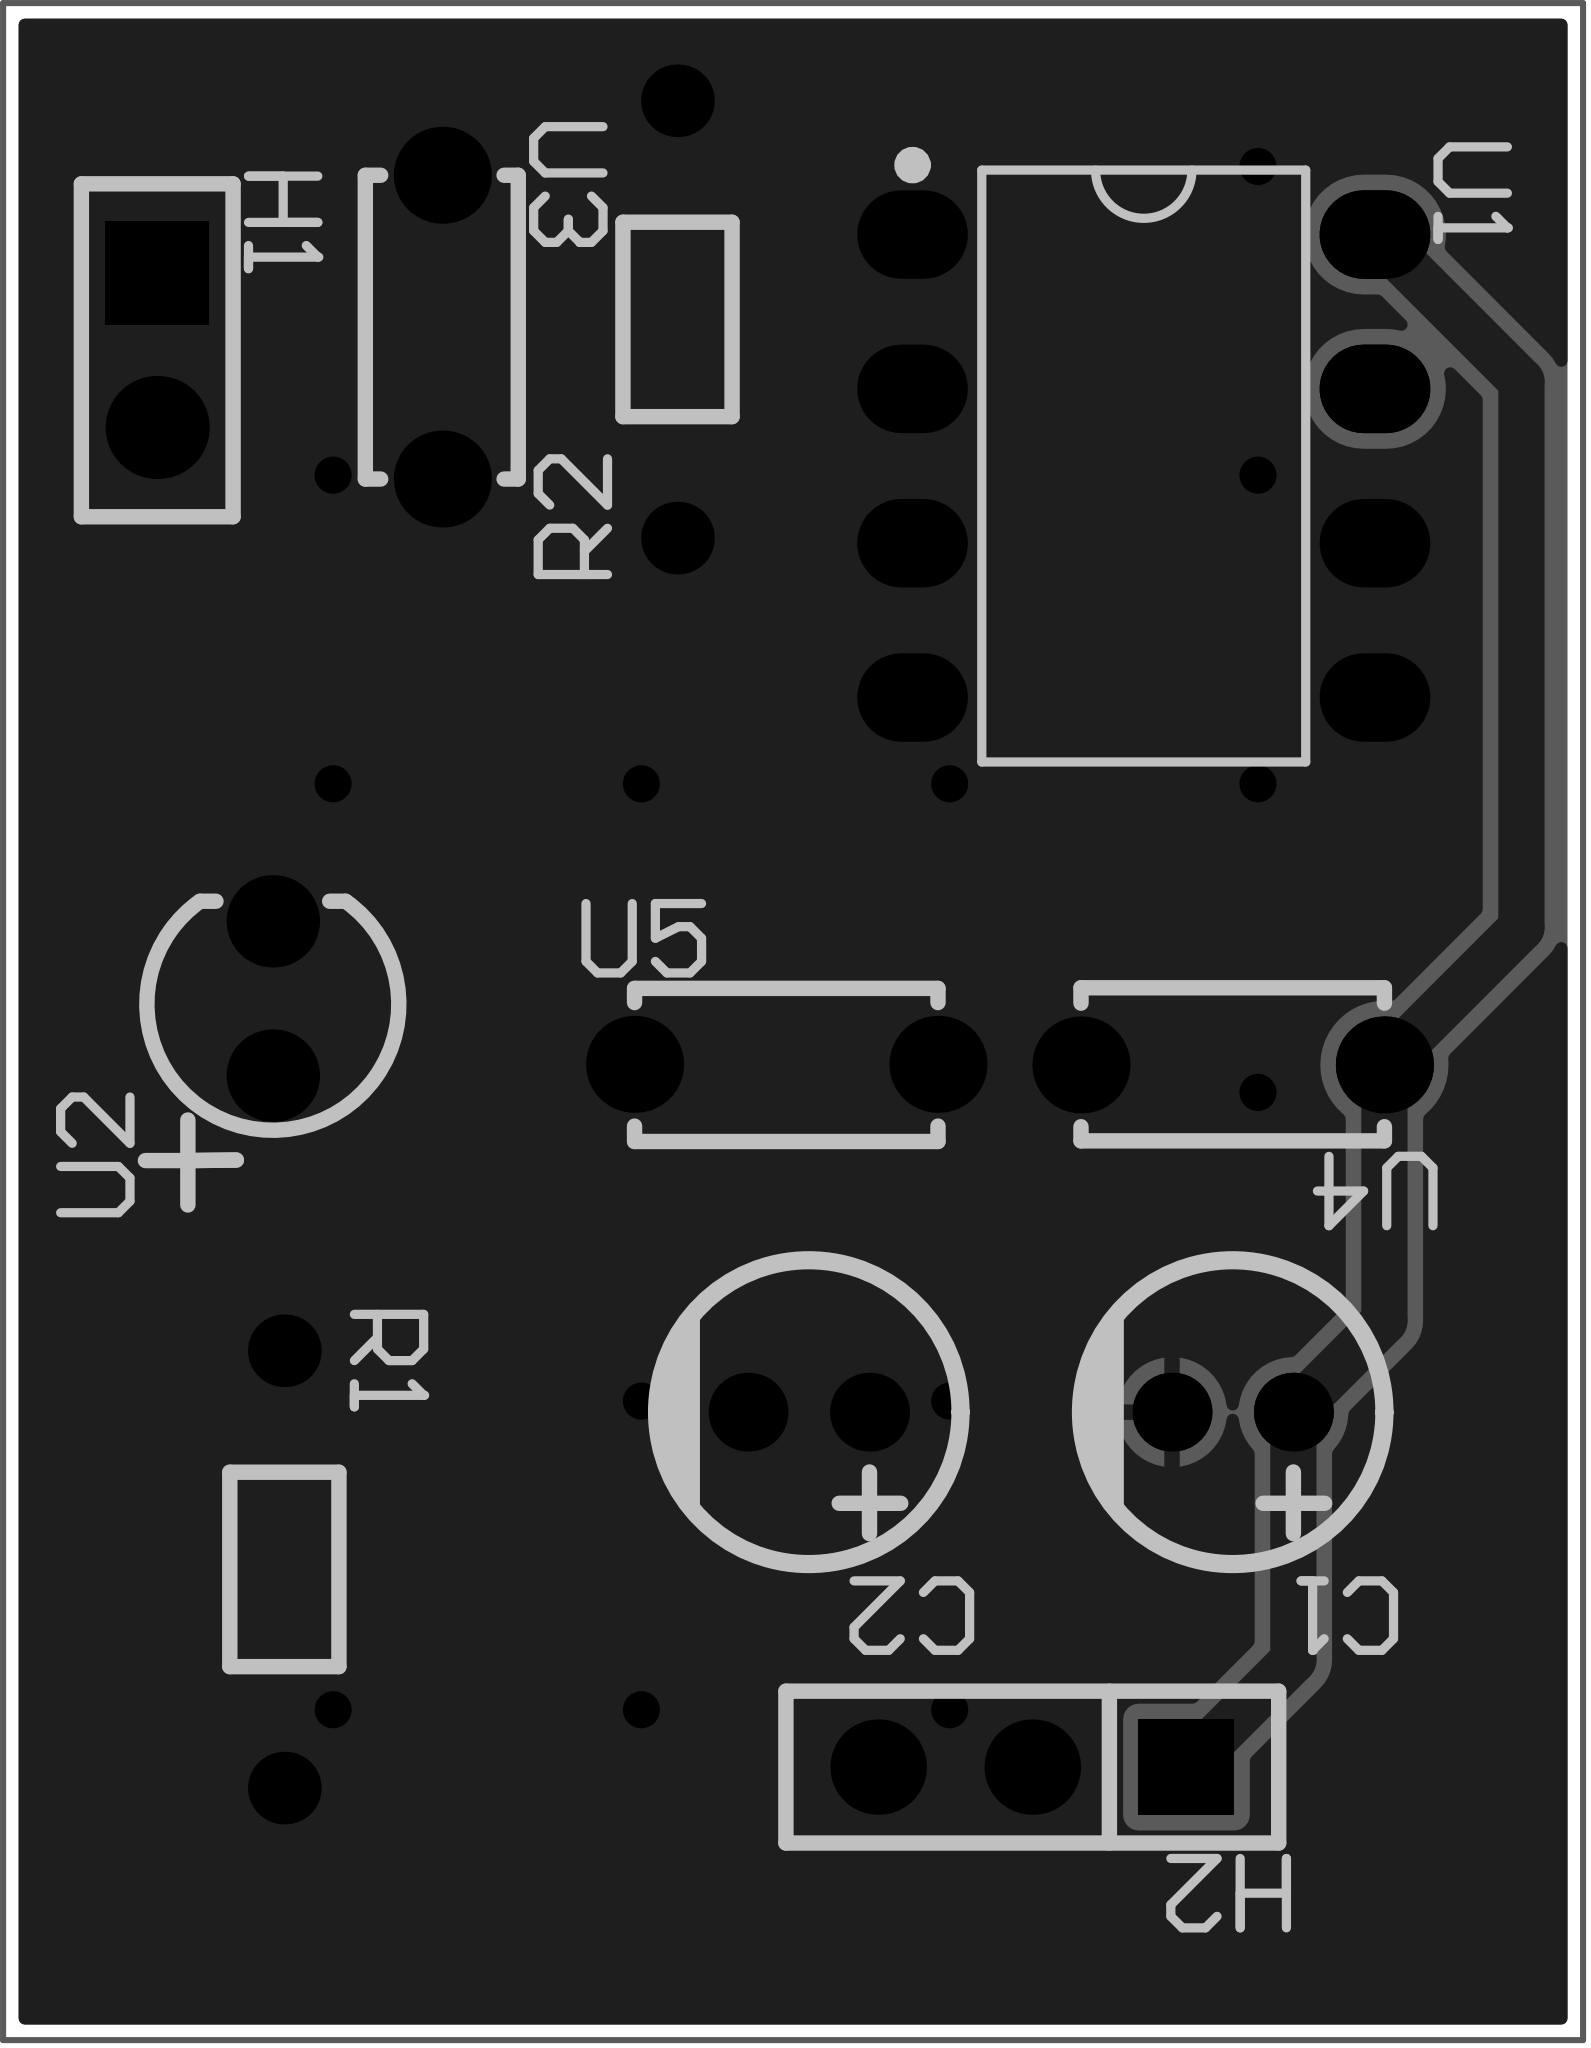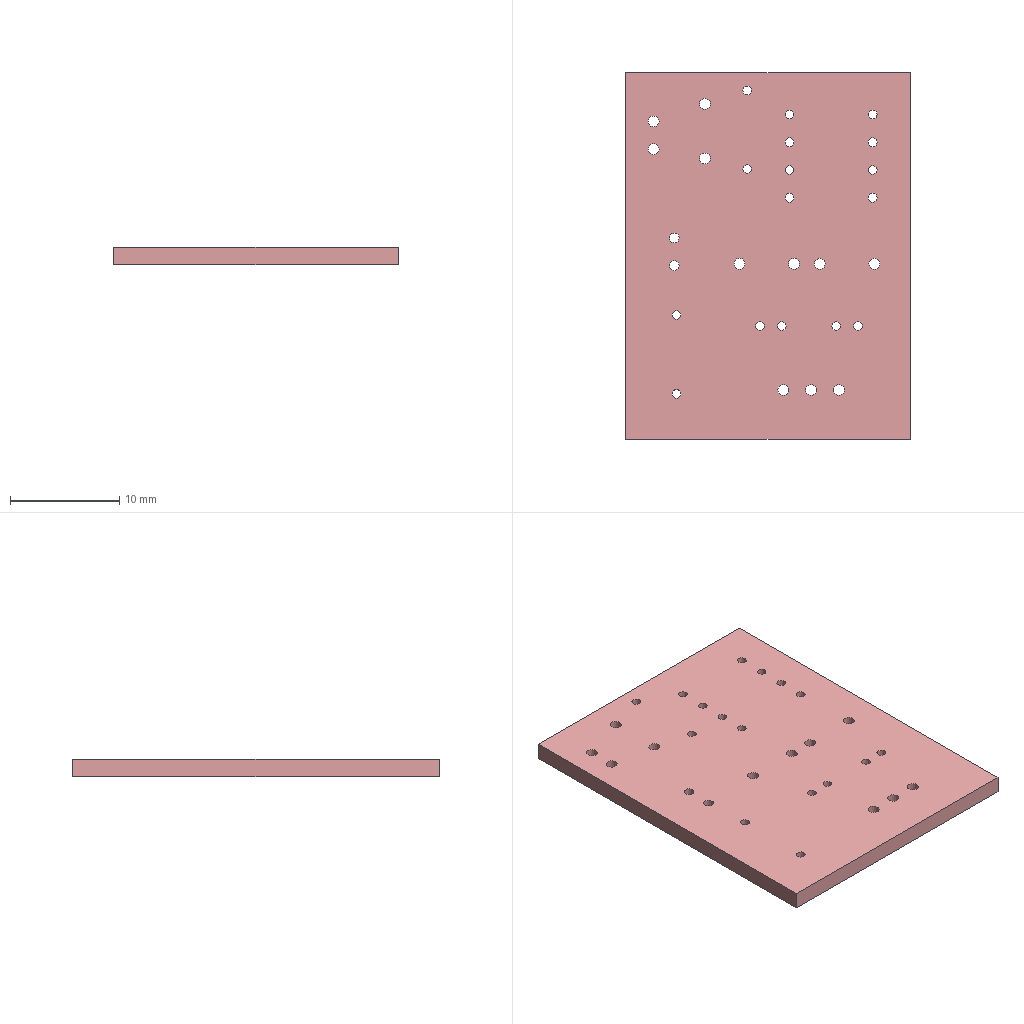Circuit board layout | Altium Designer | box 26 x 33.5 x 1.6 mm
Layer stack:
# Altium Designer layer stack of  (unit mm; dielectric type: 0 none, 1 core, 2 prepreg, 3 surface material)
index,name,kind,layer,copper_thickness_mm,dielectric_type,dielectric_thickness_mm,dielectric_material,dielectric_constant
0,Top Paste Mask Layer,other,,,,,,
1,Top Silkscreen Layer,other,,,,,,
2,Top Solder Mask Layer,dielectric,,,3,0.01,,3.3
3,Top Layer,copper,Top Layer,0.035,,,,
4,Dielectric1,dielectric,,,3,1.51,FR4,4.5
5,Bottom Layer,copper,Bottom Layer,0.035,,,,
6,Bottom Solder Mask Layer,dielectric,,,3,0.01,,3.3
7,Bottom Silkscreen Layer,other,,,,,,
8,Bottom Paste Mask Layer,other,,,,,,
# drill layer pairs: low layer,high layer
drill_pair,Top Layer,Bottom Layer
Part placement:
Designator,Comment,Layer,Footprint,Center-X(mm),Center-Y(mm),Rotation
C1,10uF,TopLayer,CAP-TH_BD5.0-P2.00-D0.8-FD-10UF50VC110GL,100.272,88.695,180
C2,10uF,TopLayer,CAP-TH_BD5.0-P2.00-D0.8-FD-10UF50VC110GL,93.287,88.695,180
H1,,TopLayer,HDR-TH_2P-P2.54-V-F,82.55,106.172,270
H2,,TopLayer,HDR-TH_3P-P2.54-V-F,96.969,82.853,180
R1,100Ω,TopLayer,Res_1/8W,84.645,86.106,270
R2,100Ω,TopLayer,Res_1/8W,91.123,106.68,90
U1,NE5532P,TopLayer,DIP-8_L9.4-W6.4-P2.54-LS9.1-BL,98.806,104.267,270
U2,SFH 4356-UV,TopLayer,LED-TH_BD3.8-P2.54-FD,84.455,95.504,90
U3,2.2pF,TopLayer,CAP-TH_L5.0-W2.5-P5.00-D1.0,87.249,106.553,270
U4,100nF,TopLayer,CAP-TH_L5.0-W2.5-P5.00-D1.0,100.272,94.409,180
U5,100nF,TopLayer,CAP-TH_L5.0-W2.5-P5.00-D1.0,92.915,94.419,0
Pad and via stacks:
# Altium Designer via and pad stacks of  (unit mm). Each distinct definition once, with the count of objects using it.
# via: kind,start_layer,end_layer,hole_mm,diameter_mm,mode(0 simple;1 top-mid-bottom;2 full stack),diameter_per_layer,count,example_net
# pad: kind,layer,hole_mm,hole_type(0 round;1 square;2 slot),plating,top_size,top_shape(1 round;2 rect;3 octagon;9 rounded rect),mid_size,bottom_size,mode,footprint,size_per_layer,count,example
pad,Multi-Layer,0.8,0,plated,1.3x1.3,1,1.3x1.3,1.3x1.3,0,CAP-TH_BD5.0-P2.00-D0.8-FD-10UF50VC110GL,,4,C1.2
pad,Multi-Layer,1,0,plated,1.7x1.7,2,1.7x1.7,1.7x1.7,0,HDR-TH_2P-P2.54-V-F,,1,H1.1
pad,Multi-Layer,1,0,plated,1.7x1.7,1,1.7x1.7,1.7x1.7,0,HDR-TH_2P-P2.54-V-F,,1,H1.2
pad,Multi-Layer,1.02,0,plated,1.575x1.575,1,1.575x1.575,1.575x1.575,0,HDR-TH_3P-P2.54-V-F,,2,H2.3
pad,Multi-Layer,1.02,0,plated,1.575x1.575,2,1.575x1.575,1.575x1.575,0,HDR-TH_3P-P2.54-V-F,,1,H2.1
pad,Multi-Layer,0.8001,0,plated,1.199x1.199,1,1.199x1.199,1.199x1.199,0,Res_1/8W,,4,R1.1
pad,Multi-Layer,0.8,0,plated,1.46x1.825,1,1.46x1.825,1.46x1.825,0,DIP-8_L9.4-W6.4-P2.54-LS9.1-BL,,8,U1.1
pad,Multi-Layer,0.9,0,plated,1.524x1.524,1,1.524x1.524,1.524x1.524,0,LED-TH_BD3.8-P2.54-FD,,2,U2.2
pad,Multi-Layer,1,0,plated,1.6x1.6,1,1.6x1.6,1.6x1.6,0,CAP-TH_L5.0-W2.5-P5.00-D1.0,,6,U3.1
via,Top Layer,Bottom Layer,0.3048,0.61,0,,13,GND
Copper pours:
name,layer,net,type(0 solid;1 hatched;2 none)
Top Layer-GND,Top Layer,GND,0
Bottom Layer-GND,Bottom Layer,GND,0
Design rules, without the lines most boards share:
# Altium Designer design rules of  (exported by Altium Designer, unit mm)
# columns: name | kind | enabled | priority | scope1 | scope2 | descriptor | typed fields (field=value)
creepage | 65 | enabled | 1 | All | All | Creepage Distance Constraint =(0mil) (All),(All) |